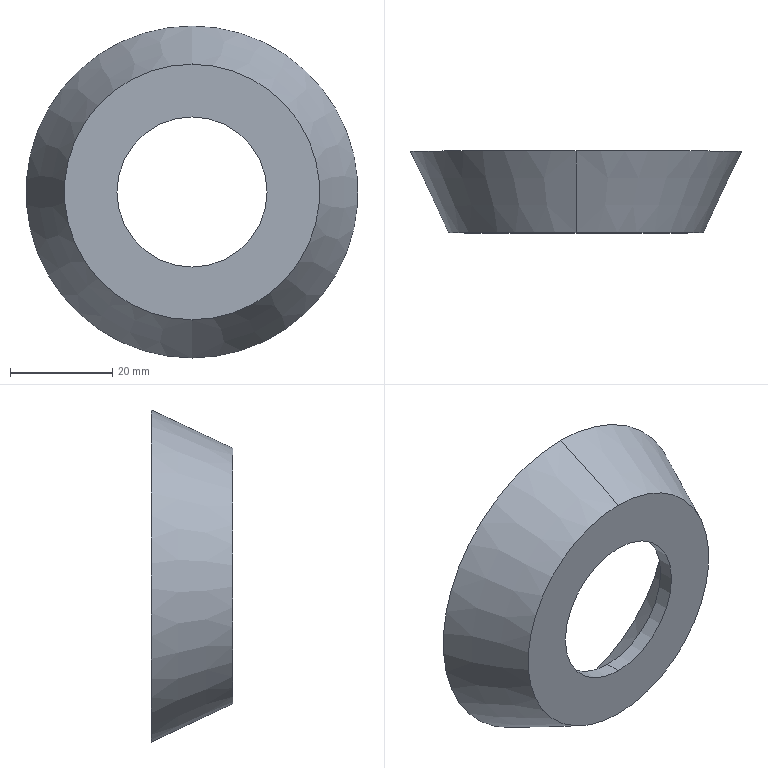Part | SolidWorks | features Revolution 1 | 1 solid | 9 faces | box 65 x 16 x 65 mm | volume 11714 mm3 | cone 4 | plane 3 | cylinder 2 | commonest cylinder face diameters 29.4 x2
STEP:
#1=CARTESIAN_POINT('',(0.,0.,25.));
#2=VERTEX_POINT('',#1);
#3=CARTESIAN_POINT('',(0.,0.,-25.));
#4=VERTEX_POINT('',#3);
#5=CARTESIAN_POINT('',(0.,0.,0.));
#6=DIRECTION('',(0.,1.,0.));
#7=DIRECTION('',(0.,0.,1.));
#8=AXIS2_PLACEMENT_3D('',#5,#6,#7);
#9=CIRCLE('',#8,25.);
#10=EDGE_CURVE('',#2,#4,#9,.T.);
#11=ORIENTED_EDGE('',*,*,#10,.T.);
#12=CARTESIAN_POINT('',(0.,16.,-32.5));
#13=VERTEX_POINT('',#12);
#14=CARTESIAN_POINT('',(0.,16.,-32.5));
#15=DIRECTION('',(0.,0.9055,-0.4244));
#16=VECTOR('',#15,1000.);
#17=LINE('',#14,#16);
#18=EDGE_CURVE('',#4,#13,#17,.T.);
#19=ORIENTED_EDGE('',*,*,#18,.T.);
#20=CARTESIAN_POINT('',(0.,16.,32.5));
#21=VERTEX_POINT('',#20);
#22=CARTESIAN_POINT('',(0.,16.,0.));
#23=DIRECTION('',(0.,1.,0.));
#24=DIRECTION('',(0.,0.,1.));
#25=AXIS2_PLACEMENT_3D('',#22,#23,#24);
#26=CIRCLE('',#25,32.5);
#27=EDGE_CURVE('',#21,#13,#26,.T.);
#28=ORIENTED_EDGE('',*,*,#27,.F.);
#29=CARTESIAN_POINT('',(0.,16.,32.5));
#30=DIRECTION('',(0.,0.9055,0.4244));
#31=VECTOR('',#30,1000.);
#32=LINE('',#29,#31);
#33=EDGE_CURVE('',#2,#21,#32,.T.);
#34=ORIENTED_EDGE('',*,*,#33,.F.);
#35=EDGE_LOOP('',(#11,#19,#28,#34));
#36=FACE_OUTER_BOUND('',#35,.T.);
#37=CARTESIAN_POINT('',(0.,16.,0.));
#38=DIRECTION('',(0.,1.,0.));
#39=DIRECTION('',(0.,0.,1.));
#40=AXIS2_PLACEMENT_3D('',#37,#38,#39);
#41=CONICAL_SURFACE('',#40,32.5,0.4383);
#42=ADVANCED_FACE('',(#36),#41,.T.);
#43=CARTESIAN_POINT('',(0.,0.,-14.7));
#44=VERTEX_POINT('',#43);
#45=CARTESIAN_POINT('',(0.,0.,14.7));
#46=VERTEX_POINT('',#45);
#47=CARTESIAN_POINT('',(0.,0.,0.));
#48=DIRECTION('',(0.,1.,0.));
#49=DIRECTION('',(0.,0.,1.));
#50=AXIS2_PLACEMENT_3D('',#47,#48,#49);
#51=CIRCLE('',#50,14.7);
#52=EDGE_CURVE('',#44,#46,#51,.T.);
#53=ORIENTED_EDGE('',*,*,#52,.F.);
#54=CARTESIAN_POINT('',(0.,3.,-14.7));
#55=VERTEX_POINT('',#54);
#56=CARTESIAN_POINT('',(0.,44.007,-14.7));
#57=DIRECTION('',(0.,1.,0.));
#58=VECTOR('',#57,1000.);
#59=LINE('',#56,#58);
#60=EDGE_CURVE('',#44,#55,#59,.T.);
#61=ORIENTED_EDGE('',*,*,#60,.T.);
#62=CARTESIAN_POINT('',(0.,3.,14.7));
#63=VERTEX_POINT('',#62);
#64=CARTESIAN_POINT('',(0.,3.,0.));
#65=DIRECTION('',(0.,1.,0.));
#66=DIRECTION('',(0.,0.,1.));
#67=AXIS2_PLACEMENT_3D('',#64,#65,#66);
#68=CIRCLE('',#67,14.7);
#69=EDGE_CURVE('',#55,#63,#68,.T.);
#70=ORIENTED_EDGE('',*,*,#69,.T.);
#71=CARTESIAN_POINT('',(0.,44.007,14.7));
#72=DIRECTION('',(0.,1.,0.));
#73=VECTOR('',#72,1000.);
#74=LINE('',#71,#73);
#75=EDGE_CURVE('',#46,#63,#74,.T.);
#76=ORIENTED_EDGE('',*,*,#75,.F.);
#77=EDGE_LOOP('',(#53,#61,#70,#76));
#78=FACE_OUTER_BOUND('',#77,.T.);
#79=CARTESIAN_POINT('',(0.,44.007,0.));
#80=DIRECTION('',(0.,1.,0.));
#81=DIRECTION('',(0.,0.,1.));
#82=AXIS2_PLACEMENT_3D('',#79,#80,#81);
#83=CYLINDRICAL_SURFACE('',#82,14.7);
#84=ADVANCED_FACE('',(#78),#83,.F.);
#85=CARTESIAN_POINT('',(0.,3.,-23.093));
#86=VERTEX_POINT('',#85);
#87=CARTESIAN_POINT('',(0.,3.,23.093));
#88=VERTEX_POINT('',#87);
#89=CARTESIAN_POINT('',(0.,3.,0.));
#90=DIRECTION('',(0.,1.,0.));
#91=DIRECTION('',(0.,0.,1.));
#92=AXIS2_PLACEMENT_3D('',#89,#90,#91);
#93=CIRCLE('',#92,23.093);
#94=EDGE_CURVE('',#86,#88,#93,.T.);
#95=ORIENTED_EDGE('',*,*,#94,.F.);
#96=CARTESIAN_POINT('',(0.,16.,-29.187));
#97=VERTEX_POINT('',#96);
#98=CARTESIAN_POINT('',(0.,3.,-23.093));
#99=DIRECTION('',(0.,0.9055,-0.4244));
#100=VECTOR('',#99,1000.);
#101=LINE('',#98,#100);
#102=EDGE_CURVE('',#86,#97,#101,.T.);
#103=ORIENTED_EDGE('',*,*,#102,.T.);
#104=CARTESIAN_POINT('',(0.,16.,29.187));
#105=VERTEX_POINT('',#104);
#106=CARTESIAN_POINT('',(0.,16.,0.));
#107=DIRECTION('',(0.,1.,0.));
#108=DIRECTION('',(0.,0.,1.));
#109=AXIS2_PLACEMENT_3D('',#106,#107,#108);
#110=CIRCLE('',#109,29.187);
#111=EDGE_CURVE('',#97,#105,#110,.T.);
#112=ORIENTED_EDGE('',*,*,#111,.T.);
#113=CARTESIAN_POINT('',(0.,3.,23.093));
#114=DIRECTION('',(0.,0.9055,0.4244));
#115=VECTOR('',#114,1000.);
#116=LINE('',#113,#115);
#117=EDGE_CURVE('',#88,#105,#116,.T.);
#118=ORIENTED_EDGE('',*,*,#117,.F.);
#119=EDGE_LOOP('',(#95,#103,#112,#118));
#120=FACE_OUTER_BOUND('',#119,.T.);
#121=CARTESIAN_POINT('',(0.,3.,0.));
#122=DIRECTION('',(0.,1.,0.));
#123=DIRECTION('',(0.,0.,1.));
#124=AXIS2_PLACEMENT_3D('',#121,#122,#123);
#125=CONICAL_SURFACE('',#124,23.093,0.4383);
#126=ADVANCED_FACE('',(#120),#125,.F.);
#127=ORIENTED_EDGE('',*,*,#27,.T.);
#128=CARTESIAN_POINT('',(0.,16.,0.));
#129=DIRECTION('',(0.,1.,0.));
#130=DIRECTION('',(0.,0.,1.));
#131=AXIS2_PLACEMENT_3D('',#128,#129,#130);
#132=CIRCLE('',#131,32.5);
#133=EDGE_CURVE('',#13,#21,#132,.T.);
#134=ORIENTED_EDGE('',*,*,#133,.T.);
#135=EDGE_LOOP('',(#127,#134));
#136=FACE_OUTER_BOUND('',#135,.T.);
#137=CARTESIAN_POINT('',(0.,16.,0.));
#138=DIRECTION('',(0.,1.,0.));
#139=DIRECTION('',(0.,0.,1.));
#140=AXIS2_PLACEMENT_3D('',#137,#138,#139);
#141=CIRCLE('',#140,29.187);
#142=EDGE_CURVE('',#105,#97,#141,.T.);
#143=ORIENTED_EDGE('',*,*,#142,.F.);
#144=ORIENTED_EDGE('',*,*,#111,.F.);
#145=EDGE_LOOP('',(#143,#144));
#146=FACE_BOUND('',#145,.T.);
#147=CARTESIAN_POINT('',(-32.5,16.,0.));
#148=DIRECTION('',(0.,1.,0.));
#149=DIRECTION('',(0.,0.,1.));
#150=AXIS2_PLACEMENT_3D('',#147,#148,#149);
#151=PLANE('',#150);
#152=ADVANCED_FACE('',(#136,#146),#151,.T.);
#153=ORIENTED_EDGE('',*,*,#102,.F.);
#154=CARTESIAN_POINT('',(0.,3.,0.));
#155=DIRECTION('',(0.,1.,0.));
#156=DIRECTION('',(0.,0.,1.));
#157=AXIS2_PLACEMENT_3D('',#154,#155,#156);
#158=CIRCLE('',#157,23.093);
#159=EDGE_CURVE('',#88,#86,#158,.T.);
#160=ORIENTED_EDGE('',*,*,#159,.F.);
#161=ORIENTED_EDGE('',*,*,#117,.T.);
#162=ORIENTED_EDGE('',*,*,#142,.T.);
#163=EDGE_LOOP('',(#153,#160,#161,#162));
#164=FACE_OUTER_BOUND('',#163,.T.);
#165=CARTESIAN_POINT('',(0.,3.,0.));
#166=DIRECTION('',(0.,1.,0.));
#167=DIRECTION('',(0.,0.,1.));
#168=AXIS2_PLACEMENT_3D('',#165,#166,#167);
#169=CONICAL_SURFACE('',#168,23.093,0.4383);
#170=ADVANCED_FACE('',(#164),#169,.F.);
#171=ORIENTED_EDGE('',*,*,#159,.T.);
#172=ORIENTED_EDGE('',*,*,#94,.T.);
#173=EDGE_LOOP('',(#171,#172));
#174=FACE_OUTER_BOUND('',#173,.T.);
#175=CARTESIAN_POINT('',(0.,3.,0.));
#176=DIRECTION('',(0.,1.,0.));
#177=DIRECTION('',(0.,0.,1.));
#178=AXIS2_PLACEMENT_3D('',#175,#176,#177);
#179=CIRCLE('',#178,14.7);
#180=EDGE_CURVE('',#63,#55,#179,.T.);
#181=ORIENTED_EDGE('',*,*,#180,.F.);
#182=ORIENTED_EDGE('',*,*,#69,.F.);
#183=EDGE_LOOP('',(#181,#182));
#184=FACE_BOUND('',#183,.T.);
#185=CARTESIAN_POINT('',(-23.093,3.,0.));
#186=DIRECTION('',(0.,1.,0.));
#187=DIRECTION('',(0.,0.,1.));
#188=AXIS2_PLACEMENT_3D('',#185,#186,#187);
#189=PLANE('',#188);
#190=ADVANCED_FACE('',(#174,#184),#189,.T.);
#191=ORIENTED_EDGE('',*,*,#60,.F.);
#192=CARTESIAN_POINT('',(0.,0.,0.));
#193=DIRECTION('',(0.,1.,0.));
#194=DIRECTION('',(0.,0.,1.));
#195=AXIS2_PLACEMENT_3D('',#192,#193,#194);
#196=CIRCLE('',#195,14.7);
#197=EDGE_CURVE('',#46,#44,#196,.T.);
#198=ORIENTED_EDGE('',*,*,#197,.F.);
#199=ORIENTED_EDGE('',*,*,#75,.T.);
#200=ORIENTED_EDGE('',*,*,#180,.T.);
#201=EDGE_LOOP('',(#191,#198,#199,#200));
#202=FACE_OUTER_BOUND('',#201,.T.);
#203=CARTESIAN_POINT('',(0.,44.007,0.));
#204=DIRECTION('',(0.,1.,0.));
#205=DIRECTION('',(0.,0.,1.));
#206=AXIS2_PLACEMENT_3D('',#203,#204,#205);
#207=CYLINDRICAL_SURFACE('',#206,14.7);
#208=ADVANCED_FACE('',(#202),#207,.F.);
#209=ORIENTED_EDGE('',*,*,#197,.T.);
#210=ORIENTED_EDGE('',*,*,#52,.T.);
#211=EDGE_LOOP('',(#209,#210));
#212=FACE_BOUND('',#211,.T.);
#213=ORIENTED_EDGE('',*,*,#10,.F.);
#214=CARTESIAN_POINT('',(0.,0.,0.));
#215=DIRECTION('',(0.,1.,0.));
#216=DIRECTION('',(0.,0.,1.));
#217=AXIS2_PLACEMENT_3D('',#214,#215,#216);
#218=CIRCLE('',#217,25.);
#219=EDGE_CURVE('',#4,#2,#218,.T.);
#220=ORIENTED_EDGE('',*,*,#219,.F.);
#221=EDGE_LOOP('',(#213,#220));
#222=FACE_OUTER_BOUND('',#221,.T.);
#223=CARTESIAN_POINT('',(-25.,0.,0.));
#224=DIRECTION('',(0.,-1.,0.));
#225=DIRECTION('',(0.,0.,-1.));
#226=AXIS2_PLACEMENT_3D('',#223,#224,#225);
#227=PLANE('',#226);
#228=ADVANCED_FACE('',(#212,#222),#227,.T.);
#229=ORIENTED_EDGE('',*,*,#18,.F.);
#230=ORIENTED_EDGE('',*,*,#219,.T.);
#231=ORIENTED_EDGE('',*,*,#33,.T.);
#232=ORIENTED_EDGE('',*,*,#133,.F.);
#233=EDGE_LOOP('',(#229,#230,#231,#232));
#234=FACE_OUTER_BOUND('',#233,.T.);
#235=CARTESIAN_POINT('',(0.,16.,0.));
#236=DIRECTION('',(0.,1.,0.));
#237=DIRECTION('',(0.,0.,1.));
#238=AXIS2_PLACEMENT_3D('',#235,#236,#237);
#239=CONICAL_SURFACE('',#238,32.5,0.4383);
#240=ADVANCED_FACE('',(#234),#239,.T.);
#241=CLOSED_SHELL('',(#42,#84,#126,#152,#170,#190,#208,#228,#240));
#242=MANIFOLD_SOLID_BREP('',#241);
#243=CARTESIAN_POINT('',(0.,0.,0.));
#244=DIRECTION('',(0.,0.,1.));
#245=DIRECTION('',(1.,0.,0.));
#246=AXIS2_PLACEMENT_3D('',#243,#244,#245);
#247=(LENGTH_UNIT()NAMED_UNIT(*)SI_UNIT(.MILLI.,.METRE.));
#248=UNCERTAINTY_MEASURE_WITH_UNIT(LENGTH_MEASURE(0.00001),#247,'','');
#249=(NAMED_UNIT(*)PLANE_ANGLE_UNIT()SI_UNIT($,.RADIAN.));
#250=(NAMED_UNIT(*)SI_UNIT($,.STERADIAN.)SOLID_ANGLE_UNIT());
#251=(GEOMETRIC_REPRESENTATION_CONTEXT(3)GLOBAL_UNCERTAINTY_ASSIGNED_CONTEXT((#248))GLOBAL_UNIT_ASSIGNED_CONTEXT((#247,#249,#250))REPRESENTATION_CONTEXT('',''));
#252=ADVANCED_BREP_SHAPE_REPRESENTATION('',(#242,#246),#251);